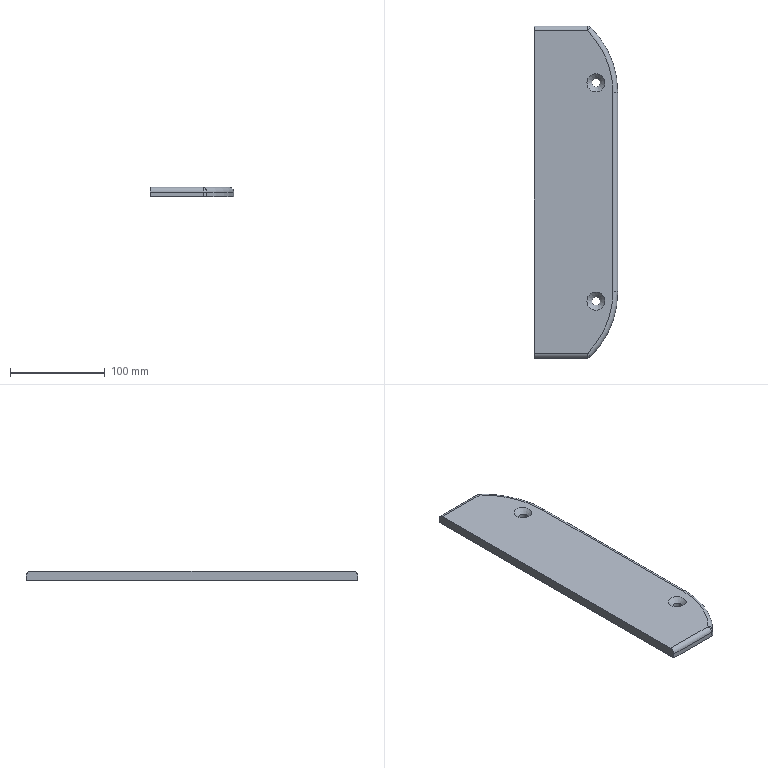Part | STEP file | Plate | 1 solid | 21 faces | box 88 x 350 x 10 mm | volume 290184 mm3 | cylinder 9 | plane 6 | cone 2 | sphere 2 | torus 2 | commonest cylinder face diameters 10 x5 9 x2 193.333 x2